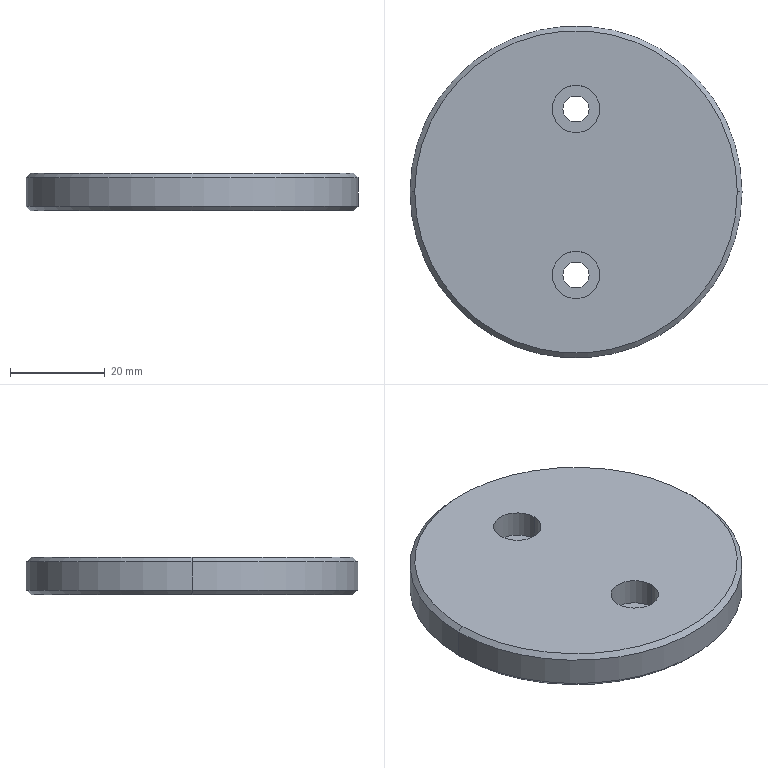Part | SolidWorks | features Chamfer 1, Extrusion 1, HoleWzd 1 | 1 solid | 18 faces | box 70 x 70 x 8 mm | volume 29565 mm3 | cylinder 10 | cone 4 | plane 4 | commonest cylinder face diameters 5.5 x4 10 x4 70 x2
STEP:
#1=CARTESIAN_POINT('',(34.,0.,8.));
#2=VERTEX_POINT('',#1);
#3=CARTESIAN_POINT('',(-34.,0.,8.));
#4=VERTEX_POINT('',#3);
#5=CARTESIAN_POINT('',(0.,0.,8.));
#6=DIRECTION('',(0.,0.,1.));
#7=DIRECTION('',(1.,0.,0.));
#8=AXIS2_PLACEMENT_3D('',#5,#6,#7);
#9=CIRCLE('',#8,34.);
#10=EDGE_CURVE('',#2,#4,#9,.T.);
#11=ORIENTED_EDGE('',*,*,#10,.F.);
#12=CARTESIAN_POINT('',(35.,0.,7.));
#13=VERTEX_POINT('',#12);
#14=CARTESIAN_POINT('',(34.,0.,8.));
#15=DIRECTION('',(0.7071,0.,-0.7071));
#16=VECTOR('',#15,1000.);
#17=LINE('',#14,#16);
#18=EDGE_CURVE('',#2,#13,#17,.T.);
#19=ORIENTED_EDGE('',*,*,#18,.T.);
#20=CARTESIAN_POINT('',(-35.,0.,7.));
#21=VERTEX_POINT('',#20);
#22=CARTESIAN_POINT('',(0.,0.,7.));
#23=DIRECTION('',(0.,0.,-1.));
#24=DIRECTION('',(1.,0.,0.));
#25=AXIS2_PLACEMENT_3D('',#22,#23,#24);
#26=CIRCLE('',#25,35.);
#27=EDGE_CURVE('',#21,#13,#26,.T.);
#28=ORIENTED_EDGE('',*,*,#27,.F.);
#29=CARTESIAN_POINT('',(-34.,0.,8.));
#30=DIRECTION('',(-0.7071,0.,-0.7071));
#31=VECTOR('',#30,1000.);
#32=LINE('',#29,#31);
#33=EDGE_CURVE('',#4,#21,#32,.T.);
#34=ORIENTED_EDGE('',*,*,#33,.F.);
#35=EDGE_LOOP('',(#11,#19,#28,#34));
#36=FACE_OUTER_BOUND('',#35,.T.);
#37=CARTESIAN_POINT('',(0.,0.,8.));
#38=DIRECTION('',(0.,0.,-1.));
#39=DIRECTION('',(-1.,0.,0.));
#40=AXIS2_PLACEMENT_3D('',#37,#38,#39);
#41=CONICAL_SURFACE('',#40,34.,0.7854);
#42=ADVANCED_FACE('',(#36),#41,.T.);
#43=CARTESIAN_POINT('',(-34.,0.,0.));
#44=VERTEX_POINT('',#43);
#45=CARTESIAN_POINT('',(34.,0.,0.));
#46=VERTEX_POINT('',#45);
#47=CARTESIAN_POINT('',(0.,0.,0.));
#48=DIRECTION('',(0.,0.,-1.));
#49=DIRECTION('',(1.,0.,0.));
#50=AXIS2_PLACEMENT_3D('',#47,#48,#49);
#51=CIRCLE('',#50,34.);
#52=EDGE_CURVE('',#44,#46,#51,.T.);
#53=ORIENTED_EDGE('',*,*,#52,.F.);
#54=CARTESIAN_POINT('',(-35.,0.,1.));
#55=VERTEX_POINT('',#54);
#56=CARTESIAN_POINT('',(-35.,0.,1.));
#57=DIRECTION('',(-0.7071,0.,0.7071));
#58=VECTOR('',#57,1000.);
#59=LINE('',#56,#58);
#60=EDGE_CURVE('',#44,#55,#59,.T.);
#61=ORIENTED_EDGE('',*,*,#60,.T.);
#62=CARTESIAN_POINT('',(35.,0.,1.));
#63=VERTEX_POINT('',#62);
#64=CARTESIAN_POINT('',(0.,0.,1.));
#65=DIRECTION('',(0.,0.,1.));
#66=DIRECTION('',(1.,0.,0.));
#67=AXIS2_PLACEMENT_3D('',#64,#65,#66);
#68=CIRCLE('',#67,35.);
#69=EDGE_CURVE('',#63,#55,#68,.T.);
#70=ORIENTED_EDGE('',*,*,#69,.F.);
#71=CARTESIAN_POINT('',(35.,0.,1.));
#72=DIRECTION('',(0.7071,0.,0.7071));
#73=VECTOR('',#72,1000.);
#74=LINE('',#71,#73);
#75=EDGE_CURVE('',#46,#63,#74,.T.);
#76=ORIENTED_EDGE('',*,*,#75,.F.);
#77=EDGE_LOOP('',(#53,#61,#70,#76));
#78=FACE_OUTER_BOUND('',#77,.T.);
#79=CARTESIAN_POINT('',(0.,0.,1.));
#80=DIRECTION('',(0.,0.,1.));
#81=DIRECTION('',(1.,0.,0.));
#82=AXIS2_PLACEMENT_3D('',#79,#80,#81);
#83=CONICAL_SURFACE('',#82,35.,0.7854);
#84=ADVANCED_FACE('',(#78),#83,.T.);
#85=CARTESIAN_POINT('',(-5.,17.5,2.3));
#86=VERTEX_POINT('',#85);
#87=CARTESIAN_POINT('',(5.,17.5,2.3));
#88=VERTEX_POINT('',#87);
#89=CARTESIAN_POINT('',(0.,17.5,2.3));
#90=DIRECTION('',(0.,0.,1.));
#91=DIRECTION('',(1.,0.,0.));
#92=AXIS2_PLACEMENT_3D('',#89,#90,#91);
#93=CIRCLE('',#92,5.);
#94=EDGE_CURVE('',#86,#88,#93,.T.);
#95=ORIENTED_EDGE('',*,*,#94,.F.);
#96=CARTESIAN_POINT('',(-5.,17.5,8.));
#97=VERTEX_POINT('',#96);
#98=CARTESIAN_POINT('',(-5.,17.5,8.));
#99=DIRECTION('',(0.,0.,1.));
#100=VECTOR('',#99,1000.);
#101=LINE('',#98,#100);
#102=EDGE_CURVE('',#86,#97,#101,.T.);
#103=ORIENTED_EDGE('',*,*,#102,.T.);
#104=CARTESIAN_POINT('',(5.,17.5,8.));
#105=VERTEX_POINT('',#104);
#106=CARTESIAN_POINT('',(0.,17.5,8.));
#107=DIRECTION('',(0.,0.,1.));
#108=DIRECTION('',(1.,0.,0.));
#109=AXIS2_PLACEMENT_3D('',#106,#107,#108);
#110=CIRCLE('',#109,5.);
#111=EDGE_CURVE('',#97,#105,#110,.T.);
#112=ORIENTED_EDGE('',*,*,#111,.T.);
#113=CARTESIAN_POINT('',(5.,17.5,8.));
#114=DIRECTION('',(0.,0.,1.));
#115=VECTOR('',#114,1000.);
#116=LINE('',#113,#115);
#117=EDGE_CURVE('',#88,#105,#116,.T.);
#118=ORIENTED_EDGE('',*,*,#117,.F.);
#119=EDGE_LOOP('',(#95,#103,#112,#118));
#120=FACE_OUTER_BOUND('',#119,.T.);
#121=CARTESIAN_POINT('',(0.,17.5,8.));
#122=DIRECTION('',(0.,0.,1.));
#123=DIRECTION('',(1.,0.,0.));
#124=AXIS2_PLACEMENT_3D('',#121,#122,#123);
#125=CYLINDRICAL_SURFACE('',#124,5.);
#126=ADVANCED_FACE('',(#120),#125,.F.);
#127=CARTESIAN_POINT('',(-2.75,17.5,0.));
#128=VERTEX_POINT('',#127);
#129=CARTESIAN_POINT('',(2.75,17.5,0.));
#130=VERTEX_POINT('',#129);
#131=CARTESIAN_POINT('',(0.,17.5,0.));
#132=DIRECTION('',(0.,0.,1.));
#133=DIRECTION('',(1.,0.,0.));
#134=AXIS2_PLACEMENT_3D('',#131,#132,#133);
#135=CIRCLE('',#134,2.75);
#136=EDGE_CURVE('',#128,#130,#135,.T.);
#137=ORIENTED_EDGE('',*,*,#136,.F.);
#138=CARTESIAN_POINT('',(-2.75,17.5,2.3));
#139=VERTEX_POINT('',#138);
#140=CARTESIAN_POINT('',(-2.75,17.5,8.));
#141=DIRECTION('',(0.,0.,1.));
#142=VECTOR('',#141,1000.);
#143=LINE('',#140,#142);
#144=EDGE_CURVE('',#128,#139,#143,.T.);
#145=ORIENTED_EDGE('',*,*,#144,.T.);
#146=CARTESIAN_POINT('',(2.75,17.5,2.3));
#147=VERTEX_POINT('',#146);
#148=CARTESIAN_POINT('',(0.,17.5,2.3));
#149=DIRECTION('',(0.,0.,1.));
#150=DIRECTION('',(1.,0.,0.));
#151=AXIS2_PLACEMENT_3D('',#148,#149,#150);
#152=CIRCLE('',#151,2.75);
#153=EDGE_CURVE('',#139,#147,#152,.T.);
#154=ORIENTED_EDGE('',*,*,#153,.T.);
#155=CARTESIAN_POINT('',(2.75,17.5,8.));
#156=DIRECTION('',(0.,0.,1.));
#157=VECTOR('',#156,1000.);
#158=LINE('',#155,#157);
#159=EDGE_CURVE('',#130,#147,#158,.T.);
#160=ORIENTED_EDGE('',*,*,#159,.F.);
#161=EDGE_LOOP('',(#137,#145,#154,#160));
#162=FACE_OUTER_BOUND('',#161,.T.);
#163=CARTESIAN_POINT('',(0.,17.5,8.));
#164=DIRECTION('',(0.,0.,1.));
#165=DIRECTION('',(1.,0.,0.));
#166=AXIS2_PLACEMENT_3D('',#163,#164,#165);
#167=CYLINDRICAL_SURFACE('',#166,2.75);
#168=ADVANCED_FACE('',(#162),#167,.F.);
#169=CARTESIAN_POINT('',(-5.,-17.5,2.3));
#170=VERTEX_POINT('',#169);
#171=CARTESIAN_POINT('',(5.,-17.5,2.3));
#172=VERTEX_POINT('',#171);
#173=CARTESIAN_POINT('',(0.,-17.5,2.3));
#174=DIRECTION('',(0.,0.,1.));
#175=DIRECTION('',(1.,0.,0.));
#176=AXIS2_PLACEMENT_3D('',#173,#174,#175);
#177=CIRCLE('',#176,5.);
#178=EDGE_CURVE('',#170,#172,#177,.T.);
#179=ORIENTED_EDGE('',*,*,#178,.F.);
#180=CARTESIAN_POINT('',(-5.,-17.5,8.));
#181=VERTEX_POINT('',#180);
#182=CARTESIAN_POINT('',(-5.,-17.5,8.));
#183=DIRECTION('',(0.,0.,1.));
#184=VECTOR('',#183,1000.);
#185=LINE('',#182,#184);
#186=EDGE_CURVE('',#170,#181,#185,.T.);
#187=ORIENTED_EDGE('',*,*,#186,.T.);
#188=CARTESIAN_POINT('',(5.,-17.5,8.));
#189=VERTEX_POINT('',#188);
#190=CARTESIAN_POINT('',(0.,-17.5,8.));
#191=DIRECTION('',(0.,0.,1.));
#192=DIRECTION('',(1.,0.,0.));
#193=AXIS2_PLACEMENT_3D('',#190,#191,#192);
#194=CIRCLE('',#193,5.);
#195=EDGE_CURVE('',#181,#189,#194,.T.);
#196=ORIENTED_EDGE('',*,*,#195,.T.);
#197=CARTESIAN_POINT('',(5.,-17.5,8.));
#198=DIRECTION('',(0.,0.,1.));
#199=VECTOR('',#198,1000.);
#200=LINE('',#197,#199);
#201=EDGE_CURVE('',#172,#189,#200,.T.);
#202=ORIENTED_EDGE('',*,*,#201,.F.);
#203=EDGE_LOOP('',(#179,#187,#196,#202));
#204=FACE_OUTER_BOUND('',#203,.T.);
#205=CARTESIAN_POINT('',(0.,-17.5,8.));
#206=DIRECTION('',(0.,0.,1.));
#207=DIRECTION('',(1.,0.,0.));
#208=AXIS2_PLACEMENT_3D('',#205,#206,#207);
#209=CYLINDRICAL_SURFACE('',#208,5.);
#210=ADVANCED_FACE('',(#204),#209,.F.);
#211=CARTESIAN_POINT('',(-2.75,-17.5,0.));
#212=VERTEX_POINT('',#211);
#213=CARTESIAN_POINT('',(2.75,-17.5,0.));
#214=VERTEX_POINT('',#213);
#215=CARTESIAN_POINT('',(0.,-17.5,0.));
#216=DIRECTION('',(0.,0.,1.));
#217=DIRECTION('',(1.,0.,0.));
#218=AXIS2_PLACEMENT_3D('',#215,#216,#217);
#219=CIRCLE('',#218,2.75);
#220=EDGE_CURVE('',#212,#214,#219,.T.);
#221=ORIENTED_EDGE('',*,*,#220,.F.);
#222=CARTESIAN_POINT('',(-2.75,-17.5,2.3));
#223=VERTEX_POINT('',#222);
#224=CARTESIAN_POINT('',(-2.75,-17.5,8.));
#225=DIRECTION('',(0.,0.,1.));
#226=VECTOR('',#225,1000.);
#227=LINE('',#224,#226);
#228=EDGE_CURVE('',#212,#223,#227,.T.);
#229=ORIENTED_EDGE('',*,*,#228,.T.);
#230=CARTESIAN_POINT('',(2.75,-17.5,2.3));
#231=VERTEX_POINT('',#230);
#232=CARTESIAN_POINT('',(0.,-17.5,2.3));
#233=DIRECTION('',(0.,0.,1.));
#234=DIRECTION('',(1.,0.,0.));
#235=AXIS2_PLACEMENT_3D('',#232,#233,#234);
#236=CIRCLE('',#235,2.75);
#237=EDGE_CURVE('',#223,#231,#236,.T.);
#238=ORIENTED_EDGE('',*,*,#237,.T.);
#239=CARTESIAN_POINT('',(2.75,-17.5,8.));
#240=DIRECTION('',(0.,0.,1.));
#241=VECTOR('',#240,1000.);
#242=LINE('',#239,#241);
#243=EDGE_CURVE('',#214,#231,#242,.T.);
#244=ORIENTED_EDGE('',*,*,#243,.F.);
#245=EDGE_LOOP('',(#221,#229,#238,#244));
#246=FACE_OUTER_BOUND('',#245,.T.);
#247=CARTESIAN_POINT('',(0.,-17.5,8.));
#248=DIRECTION('',(0.,0.,1.));
#249=DIRECTION('',(1.,0.,0.));
#250=AXIS2_PLACEMENT_3D('',#247,#248,#249);
#251=CYLINDRICAL_SURFACE('',#250,2.75);
#252=ADVANCED_FACE('',(#246),#251,.F.);
#253=ORIENTED_EDGE('',*,*,#27,.T.);
#254=CARTESIAN_POINT('',(35.,0.,8.));
#255=DIRECTION('',(0.,0.,-1.));
#256=VECTOR('',#255,1000.);
#257=LINE('',#254,#256);
#258=EDGE_CURVE('',#13,#63,#257,.T.);
#259=ORIENTED_EDGE('',*,*,#258,.T.);
#260=ORIENTED_EDGE('',*,*,#69,.T.);
#261=CARTESIAN_POINT('',(-35.,0.,8.));
#262=DIRECTION('',(0.,0.,-1.));
#263=VECTOR('',#262,1000.);
#264=LINE('',#261,#263);
#265=EDGE_CURVE('',#21,#55,#264,.T.);
#266=ORIENTED_EDGE('',*,*,#265,.F.);
#267=EDGE_LOOP('',(#253,#259,#260,#266));
#268=FACE_OUTER_BOUND('',#267,.T.);
#269=CARTESIAN_POINT('',(0.,0.,8.));
#270=DIRECTION('',(0.,0.,-1.));
#271=DIRECTION('',(-1.,0.,0.));
#272=AXIS2_PLACEMENT_3D('',#269,#270,#271);
#273=CYLINDRICAL_SURFACE('',#272,35.);
#274=ADVANCED_FACE('',(#268),#273,.T.);
#275=ORIENTED_EDGE('',*,*,#258,.F.);
#276=CARTESIAN_POINT('',(0.,0.,7.));
#277=DIRECTION('',(0.,0.,-1.));
#278=DIRECTION('',(1.,0.,0.));
#279=AXIS2_PLACEMENT_3D('',#276,#277,#278);
#280=CIRCLE('',#279,35.);
#281=EDGE_CURVE('',#13,#21,#280,.T.);
#282=ORIENTED_EDGE('',*,*,#281,.T.);
#283=ORIENTED_EDGE('',*,*,#265,.T.);
#284=CARTESIAN_POINT('',(0.,0.,1.));
#285=DIRECTION('',(0.,0.,1.));
#286=DIRECTION('',(1.,0.,0.));
#287=AXIS2_PLACEMENT_3D('',#284,#285,#286);
#288=CIRCLE('',#287,35.);
#289=EDGE_CURVE('',#55,#63,#288,.T.);
#290=ORIENTED_EDGE('',*,*,#289,.T.);
#291=EDGE_LOOP('',(#275,#282,#283,#290));
#292=FACE_OUTER_BOUND('',#291,.T.);
#293=CARTESIAN_POINT('',(0.,0.,8.));
#294=DIRECTION('',(0.,0.,-1.));
#295=DIRECTION('',(-1.,0.,0.));
#296=AXIS2_PLACEMENT_3D('',#293,#294,#295);
#297=CYLINDRICAL_SURFACE('',#296,35.);
#298=ADVANCED_FACE('',(#292),#297,.T.);
#299=CARTESIAN_POINT('',(0.,0.,8.));
#300=DIRECTION('',(0.,0.,1.));
#301=DIRECTION('',(1.,0.,0.));
#302=AXIS2_PLACEMENT_3D('',#299,#300,#301);
#303=CIRCLE('',#302,34.);
#304=EDGE_CURVE('',#4,#2,#303,.T.);
#305=ORIENTED_EDGE('',*,*,#304,.T.);
#306=ORIENTED_EDGE('',*,*,#10,.T.);
#307=EDGE_LOOP('',(#305,#306));
#308=FACE_OUTER_BOUND('',#307,.T.);
#309=CARTESIAN_POINT('',(0.,17.5,8.));
#310=DIRECTION('',(0.,0.,1.));
#311=DIRECTION('',(1.,0.,0.));
#312=AXIS2_PLACEMENT_3D('',#309,#310,#311);
#313=CIRCLE('',#312,5.);
#314=EDGE_CURVE('',#105,#97,#313,.T.);
#315=ORIENTED_EDGE('',*,*,#314,.F.);
#316=ORIENTED_EDGE('',*,*,#111,.F.);
#317=EDGE_LOOP('',(#315,#316));
#318=FACE_BOUND('',#317,.T.);
#319=CARTESIAN_POINT('',(0.,-17.5,8.));
#320=DIRECTION('',(0.,0.,1.));
#321=DIRECTION('',(1.,0.,0.));
#322=AXIS2_PLACEMENT_3D('',#319,#320,#321);
#323=CIRCLE('',#322,5.);
#324=EDGE_CURVE('',#189,#181,#323,.T.);
#325=ORIENTED_EDGE('',*,*,#324,.F.);
#326=ORIENTED_EDGE('',*,*,#195,.F.);
#327=EDGE_LOOP('',(#325,#326));
#328=FACE_BOUND('',#327,.T.);
#329=CARTESIAN_POINT('',(0.,0.,8.));
#330=DIRECTION('',(0.,0.,1.));
#331=DIRECTION('',(1.,0.,0.));
#332=AXIS2_PLACEMENT_3D('',#329,#330,#331);
#333=PLANE('',#332);
#334=ADVANCED_FACE('',(#308,#318,#328),#333,.T.);
#335=CARTESIAN_POINT('',(0.,0.,0.));
#336=DIRECTION('',(0.,0.,-1.));
#337=DIRECTION('',(1.,0.,0.));
#338=AXIS2_PLACEMENT_3D('',#335,#336,#337);
#339=CIRCLE('',#338,34.);
#340=EDGE_CURVE('',#46,#44,#339,.T.);
#341=ORIENTED_EDGE('',*,*,#340,.T.);
#342=ORIENTED_EDGE('',*,*,#52,.T.);
#343=EDGE_LOOP('',(#341,#342));
#344=FACE_OUTER_BOUND('',#343,.T.);
#345=CARTESIAN_POINT('',(0.,17.5,0.));
#346=DIRECTION('',(0.,0.,1.));
#347=DIRECTION('',(1.,0.,0.));
#348=AXIS2_PLACEMENT_3D('',#345,#346,#347);
#349=CIRCLE('',#348,2.75);
#350=EDGE_CURVE('',#130,#128,#349,.T.);
#351=ORIENTED_EDGE('',*,*,#350,.T.);
#352=ORIENTED_EDGE('',*,*,#136,.T.);
#353=EDGE_LOOP('',(#351,#352));
#354=FACE_BOUND('',#353,.T.);
#355=CARTESIAN_POINT('',(0.,-17.5,0.));
#356=DIRECTION('',(0.,0.,1.));
#357=DIRECTION('',(1.,0.,0.));
#358=AXIS2_PLACEMENT_3D('',#355,#356,#357);
#359=CIRCLE('',#358,2.75);
#360=EDGE_CURVE('',#214,#212,#359,.T.);
#361=ORIENTED_EDGE('',*,*,#360,.T.);
#362=ORIENTED_EDGE('',*,*,#220,.T.);
#363=EDGE_LOOP('',(#361,#362));
#364=FACE_BOUND('',#363,.T.);
#365=CARTESIAN_POINT('',(0.,0.,0.));
#366=DIRECTION('',(0.,0.,1.));
#367=DIRECTION('',(1.,0.,0.));
#368=AXIS2_PLACEMENT_3D('',#365,#366,#367);
#369=PLANE('',#368);
#370=ADVANCED_FACE('',(#344,#354,#364),#369,.F.);
#371=ORIENTED_EDGE('',*,*,#228,.F.);
#372=ORIENTED_EDGE('',*,*,#360,.F.);
#373=ORIENTED_EDGE('',*,*,#243,.T.);
#374=CARTESIAN_POINT('',(0.,-17.5,2.3));
#375=DIRECTION('',(0.,0.,1.));
#376=DIRECTION('',(1.,0.,0.));
#377=AXIS2_PLACEMENT_3D('',#374,#375,#376);
#378=CIRCLE('',#377,2.75);
#379=EDGE_CURVE('',#231,#223,#378,.T.);
#380=ORIENTED_EDGE('',*,*,#379,.T.);
#381=EDGE_LOOP('',(#371,#372,#373,#380));
#382=FACE_OUTER_BOUND('',#381,.T.);
#383=CARTESIAN_POINT('',(0.,-17.5,8.));
#384=DIRECTION('',(0.,0.,1.));
#385=DIRECTION('',(1.,0.,0.));
#386=AXIS2_PLACEMENT_3D('',#383,#384,#385);
#387=CYLINDRICAL_SURFACE('',#386,2.75);
#388=ADVANCED_FACE('',(#382),#387,.F.);
#389=ORIENTED_EDGE('',*,*,#379,.F.);
#390=ORIENTED_EDGE('',*,*,#237,.F.);
#391=EDGE_LOOP('',(#389,#390));
#392=FACE_BOUND('',#391,.T.);
#393=CARTESIAN_POINT('',(0.,-17.5,2.3));
#394=DIRECTION('',(0.,0.,1.));
#395=DIRECTION('',(1.,0.,0.));
#396=AXIS2_PLACEMENT_3D('',#393,#394,#395);
#397=CIRCLE('',#396,5.);
#398=EDGE_CURVE('',#172,#170,#397,.T.);
#399=ORIENTED_EDGE('',*,*,#398,.T.);
#400=ORIENTED_EDGE('',*,*,#178,.T.);
#401=EDGE_LOOP('',(#399,#400));
#402=FACE_OUTER_BOUND('',#401,.T.);
#403=CARTESIAN_POINT('',(2.75,-17.5,2.3));
#404=DIRECTION('',(0.,0.,-1.));
#405=DIRECTION('',(-1.,0.,0.));
#406=AXIS2_PLACEMENT_3D('',#403,#404,#405);
#407=PLANE('',#406);
#408=ADVANCED_FACE('',(#392,#402),#407,.F.);
#409=ORIENTED_EDGE('',*,*,#186,.F.);
#410=ORIENTED_EDGE('',*,*,#398,.F.);
#411=ORIENTED_EDGE('',*,*,#201,.T.);
#412=ORIENTED_EDGE('',*,*,#324,.T.);
#413=EDGE_LOOP('',(#409,#410,#411,#412));
#414=FACE_OUTER_BOUND('',#413,.T.);
#415=CARTESIAN_POINT('',(0.,-17.5,8.));
#416=DIRECTION('',(0.,0.,1.));
#417=DIRECTION('',(1.,0.,0.));
#418=AXIS2_PLACEMENT_3D('',#415,#416,#417);
#419=CYLINDRICAL_SURFACE('',#418,5.);
#420=ADVANCED_FACE('',(#414),#419,.F.);
#421=ORIENTED_EDGE('',*,*,#144,.F.);
#422=ORIENTED_EDGE('',*,*,#350,.F.);
#423=ORIENTED_EDGE('',*,*,#159,.T.);
#424=CARTESIAN_POINT('',(0.,17.5,2.3));
#425=DIRECTION('',(0.,0.,1.));
#426=DIRECTION('',(1.,0.,0.));
#427=AXIS2_PLACEMENT_3D('',#424,#425,#426);
#428=CIRCLE('',#427,2.75);
#429=EDGE_CURVE('',#147,#139,#428,.T.);
#430=ORIENTED_EDGE('',*,*,#429,.T.);
#431=EDGE_LOOP('',(#421,#422,#423,#430));
#432=FACE_OUTER_BOUND('',#431,.T.);
#433=CARTESIAN_POINT('',(0.,17.5,8.));
#434=DIRECTION('',(0.,0.,1.));
#435=DIRECTION('',(1.,0.,0.));
#436=AXIS2_PLACEMENT_3D('',#433,#434,#435);
#437=CYLINDRICAL_SURFACE('',#436,2.75);
#438=ADVANCED_FACE('',(#432),#437,.F.);
#439=ORIENTED_EDGE('',*,*,#429,.F.);
#440=ORIENTED_EDGE('',*,*,#153,.F.);
#441=EDGE_LOOP('',(#439,#440));
#442=FACE_BOUND('',#441,.T.);
#443=CARTESIAN_POINT('',(0.,17.5,2.3));
#444=DIRECTION('',(0.,0.,1.));
#445=DIRECTION('',(1.,0.,0.));
#446=AXIS2_PLACEMENT_3D('',#443,#444,#445);
#447=CIRCLE('',#446,5.);
#448=EDGE_CURVE('',#88,#86,#447,.T.);
#449=ORIENTED_EDGE('',*,*,#448,.T.);
#450=ORIENTED_EDGE('',*,*,#94,.T.);
#451=EDGE_LOOP('',(#449,#450));
#452=FACE_OUTER_BOUND('',#451,.T.);
#453=CARTESIAN_POINT('',(2.75,17.5,2.3));
#454=DIRECTION('',(0.,0.,-1.));
#455=DIRECTION('',(-1.,0.,0.));
#456=AXIS2_PLACEMENT_3D('',#453,#454,#455);
#457=PLANE('',#456);
#458=ADVANCED_FACE('',(#442,#452),#457,.F.);
#459=ORIENTED_EDGE('',*,*,#102,.F.);
#460=ORIENTED_EDGE('',*,*,#448,.F.);
#461=ORIENTED_EDGE('',*,*,#117,.T.);
#462=ORIENTED_EDGE('',*,*,#314,.T.);
#463=EDGE_LOOP('',(#459,#460,#461,#462));
#464=FACE_OUTER_BOUND('',#463,.T.);
#465=CARTESIAN_POINT('',(0.,17.5,8.));
#466=DIRECTION('',(0.,0.,1.));
#467=DIRECTION('',(1.,0.,0.));
#468=AXIS2_PLACEMENT_3D('',#465,#466,#467);
#469=CYLINDRICAL_SURFACE('',#468,5.);
#470=ADVANCED_FACE('',(#464),#469,.F.);
#471=ORIENTED_EDGE('',*,*,#60,.F.);
#472=ORIENTED_EDGE('',*,*,#340,.F.);
#473=ORIENTED_EDGE('',*,*,#75,.T.);
#474=ORIENTED_EDGE('',*,*,#289,.F.);
#475=EDGE_LOOP('',(#471,#472,#473,#474));
#476=FACE_OUTER_BOUND('',#475,.T.);
#477=CARTESIAN_POINT('',(0.,0.,1.));
#478=DIRECTION('',(0.,0.,1.));
#479=DIRECTION('',(1.,0.,0.));
#480=AXIS2_PLACEMENT_3D('',#477,#478,#479);
#481=CONICAL_SURFACE('',#480,35.,0.7854);
#482=ADVANCED_FACE('',(#476),#481,.T.);
#483=ORIENTED_EDGE('',*,*,#18,.F.);
#484=ORIENTED_EDGE('',*,*,#304,.F.);
#485=ORIENTED_EDGE('',*,*,#33,.T.);
#486=ORIENTED_EDGE('',*,*,#281,.F.);
#487=EDGE_LOOP('',(#483,#484,#485,#486));
#488=FACE_OUTER_BOUND('',#487,.T.);
#489=CARTESIAN_POINT('',(0.,0.,8.));
#490=DIRECTION('',(0.,0.,-1.));
#491=DIRECTION('',(-1.,0.,0.));
#492=AXIS2_PLACEMENT_3D('',#489,#490,#491);
#493=CONICAL_SURFACE('',#492,34.,0.7854);
#494=ADVANCED_FACE('',(#488),#493,.T.);
#495=CLOSED_SHELL('',(#42,#84,#126,#168,#210,#252,#274,#298,#334,#370,#388,#408,#420,#438,#458,#470,#482,#494));
#496=MANIFOLD_SOLID_BREP('',#495);
#497=CARTESIAN_POINT('',(0.,0.,0.));
#498=DIRECTION('',(0.,0.,1.));
#499=DIRECTION('',(1.,0.,0.));
#500=AXIS2_PLACEMENT_3D('',#497,#498,#499);
#501=(LENGTH_UNIT()NAMED_UNIT(*)SI_UNIT(.MILLI.,.METRE.));
#502=UNCERTAINTY_MEASURE_WITH_UNIT(LENGTH_MEASURE(0.00001),#501,'','');
#503=(NAMED_UNIT(*)PLANE_ANGLE_UNIT()SI_UNIT($,.RADIAN.));
#504=(NAMED_UNIT(*)SI_UNIT($,.STERADIAN.)SOLID_ANGLE_UNIT());
#505=(GEOMETRIC_REPRESENTATION_CONTEXT(3)GLOBAL_UNCERTAINTY_ASSIGNED_CONTEXT((#502))GLOBAL_UNIT_ASSIGNED_CONTEXT((#501,#503,#504))REPRESENTATION_CONTEXT('',''));
#506=ADVANCED_BREP_SHAPE_REPRESENTATION('',(#496,#500),#505);